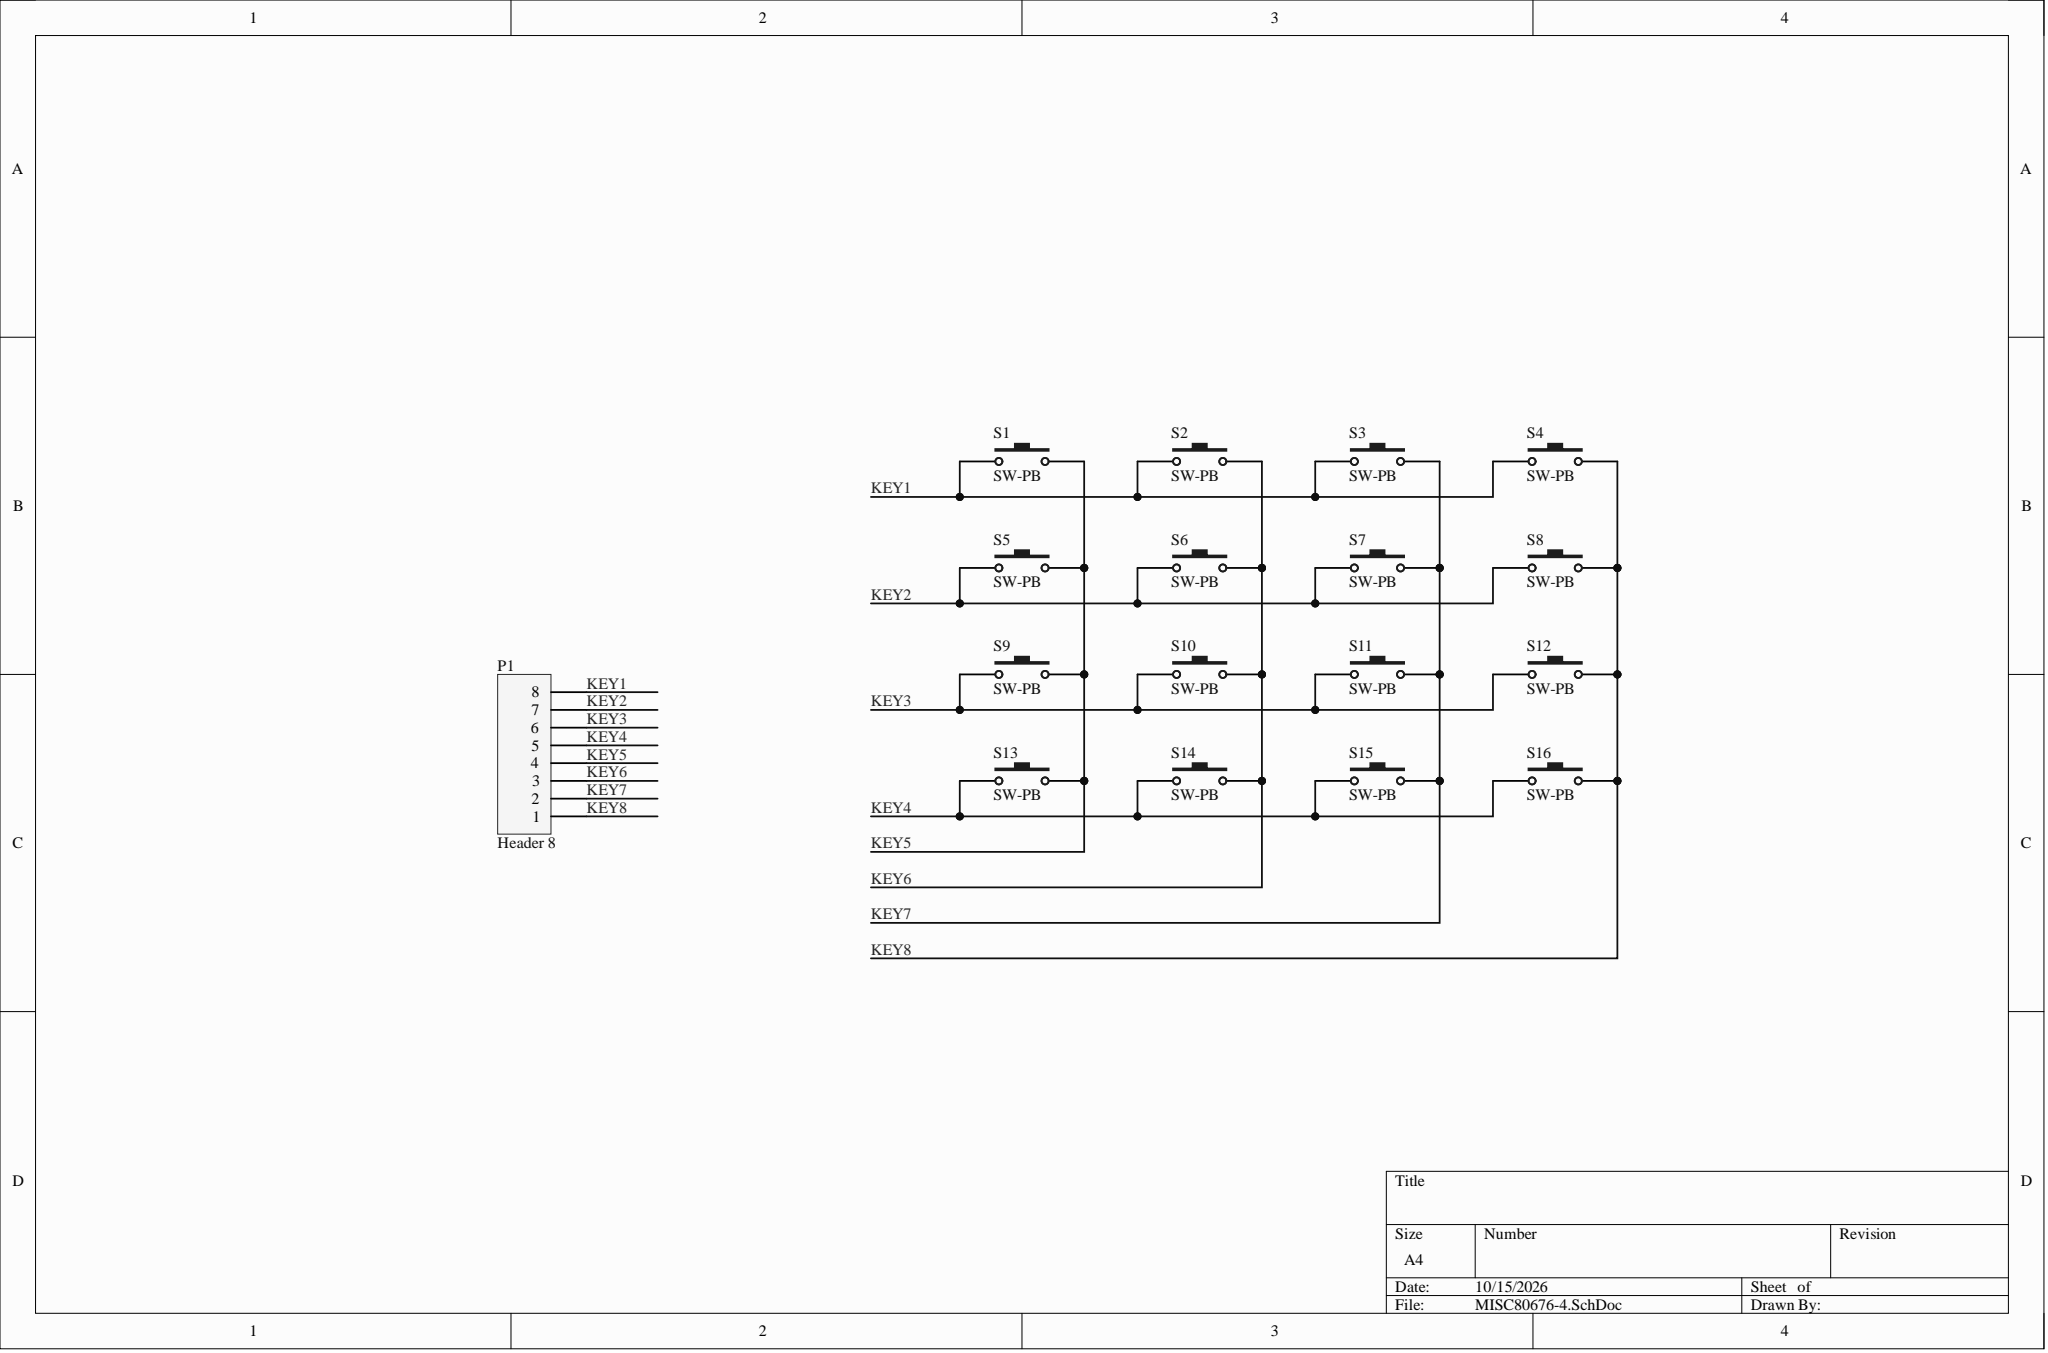Circuit board | Altium Designer | 17 parts | 8 nets
Bill of materials:
Comment,Description,Designator,Footprint,LibRef,Quantity
"Header 8","Header, 8-Pin","P1","HDR1X8","Header 8","1"
"SW-PB","Switch","S1, S2, S3, S4, S5, S6, S7, S8, S9, S10, S11, S12, S13, S14, S15, S16","SPST-2","SW-PB","16"
Netlist (Protel format):
[
P1
HDR1X8
Header 8



]
[
S1
SPST-2
SW-PB



]
[
S2
SPST-2
SW-PB



]
[
S3
SPST-2
SW-PB



]
[
S4
SPST-2
SW-PB



]
[
S5
SPST-2
SW-PB



]
[
S6
SPST-2
SW-PB



]
[
S7
SPST-2
SW-PB



]
[
S8
SPST-2
SW-PB



]
[
S9
SPST-2
SW-PB



]
[
S10
SPST-2
SW-PB



]
[
S11
SPST-2
SW-PB



]
[
S12
SPST-2
SW-PB



]
[
S13
SPST-2
SW-PB



]
[
S14
SPST-2
SW-PB



]
[
S15
SPST-2
SW-PB



]
[
S16
SPST-2
SW-PB



]
(
KEY8
P1-1
S4-2
S8-2
S12-2
S16-2
)
(
KEY7
P1-2
S3-2
S7-2
S11-2
S15-2
)
(
KEY6
P1-3
S2-2
S6-2
S10-2
S14-2
)
(
KEY5
P1-4
S1-2
S5-2
S9-2
S13-2
)
(
KEY4
P1-5
S13-1
S14-1
S15-1
S16-1
)
(
KEY3
P1-6
S9-1
S10-1
S11-1
S12-1
)
(
KEY2
P1-7
S5-1
S6-1
S7-1
S8-1
)
(
KEY1
P1-8
S1-1
S2-1
S3-1
S4-1
)